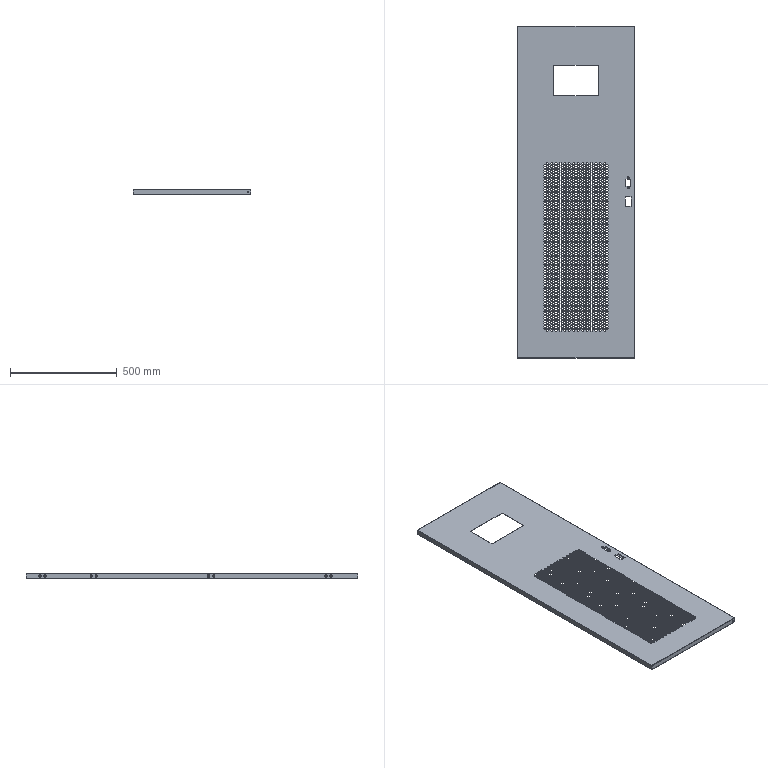Part | SolidWorks | features APattern 1, ICE 1, SplitBody 1 | 1 solid | 11548 faces | volume 997556 mm3 | plane 11460 | cylinder 72 | spline 16 | commonest cylinder face diameters 5.5 x16 6.5 x16 11.5 x16 0.2 x8 2.6 x8 4.5 x4